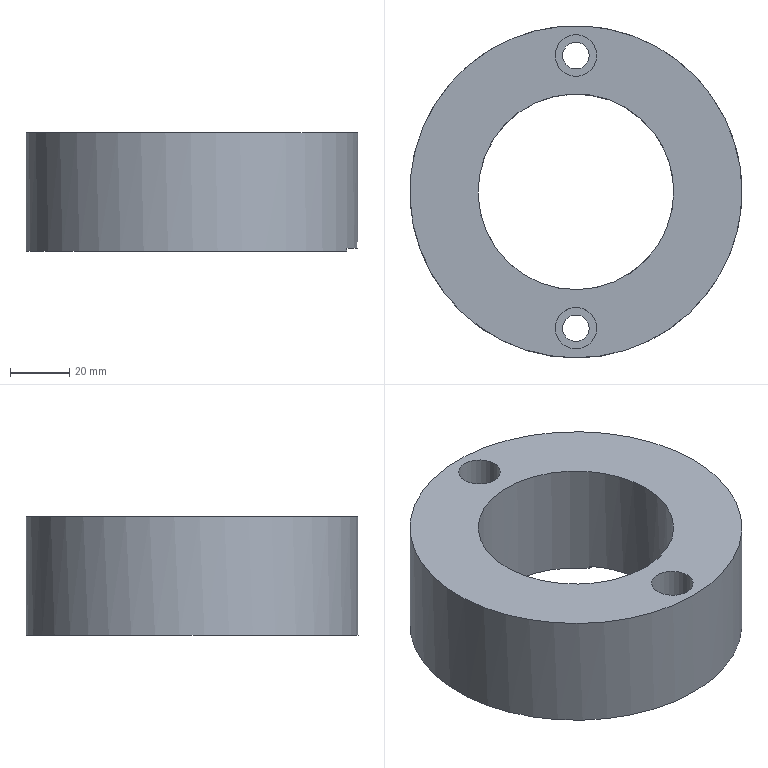Part | NX | features solid 2 | 1 solid | 13 faces | box 112 x 112 x 40 mm | volume 247574 mm3 | plane 7 | cylinder 6 | commonest cylinder face diameters 9 x2 14 x2 66 x1 112 x1
STEP:
#1=CARTESIAN_POINT('',(-633.751,-130.,-30.));
#2=VERTEX_POINT('',#1);
#3=CARTESIAN_POINT('',(-633.751,-130.,-29.));
#4=VERTEX_POINT('',#3);
#5=CARTESIAN_POINT('',(-633.751,-130.,20.));
#6=DIRECTION('',(0.,0.,-1.));
#7=VECTOR('',#6,1000.);
#8=LINE('',#5,#7);
#9=EDGE_CURVE('',#2,#4,#8,.F.);
#10=ORIENTED_EDGE('',*,*,#9,.T.);
#11=CARTESIAN_POINT('',(-633.751,-170.,-29.));
#12=VERTEX_POINT('',#11);
#13=CARTESIAN_POINT('',(-660.,-150.,-29.));
#14=DIRECTION('',(0.,0.,-1.));
#15=DIRECTION('',(1.,0.,0.));
#16=AXIS2_PLACEMENT_3D('',#13,#14,#15);
#17=CIRCLE('',#16,33.);
#18=EDGE_CURVE('',#4,#12,#17,.T.);
#19=ORIENTED_EDGE('',*,*,#18,.T.);
#20=CARTESIAN_POINT('',(-633.751,-170.,-30.));
#21=VERTEX_POINT('',#20);
#22=CARTESIAN_POINT('',(-633.751,-170.,20.));
#23=DIRECTION('',(0.,0.,-1.));
#24=VECTOR('',#23,1000.);
#25=LINE('',#22,#24);
#26=EDGE_CURVE('',#12,#21,#25,.T.);
#27=ORIENTED_EDGE('',*,*,#26,.T.);
#28=CARTESIAN_POINT('',(-660.,-150.,-30.));
#29=DIRECTION('',(0.,0.,-1.));
#30=DIRECTION('',(1.,0.,0.));
#31=AXIS2_PLACEMENT_3D('',#28,#29,#30);
#32=CIRCLE('',#31,33.);
#33=EDGE_CURVE('',#21,#2,#32,.T.);
#34=ORIENTED_EDGE('',*,*,#33,.T.);
#35=EDGE_LOOP('',(#10,#19,#27,#34));
#36=FACE_BOUND('',#35,.T.);
#37=CARTESIAN_POINT('',(-627.,-150.,10.));
#38=VERTEX_POINT('',#37);
#39=CARTESIAN_POINT('',(-660.,-150.,10.));
#40=DIRECTION('',(0.,0.,-1.));
#41=DIRECTION('',(1.,0.,0.));
#42=AXIS2_PLACEMENT_3D('',#39,#40,#41);
#43=CIRCLE('',#42,33.);
#44=EDGE_CURVE('',#38,#38,#43,.T.);
#45=ORIENTED_EDGE('',*,*,#44,.F.);
#46=EDGE_LOOP('',(#45));
#47=FACE_BOUND('',#46,.T.);
#48=CARTESIAN_POINT('',(-660.,-150.,20.));
#49=DIRECTION('',(0.,0.,-1.));
#50=DIRECTION('',(-1.,0.,0.));
#51=AXIS2_PLACEMENT_3D('',#48,#49,#50);
#52=CYLINDRICAL_SURFACE('',#51,33.);
#53=ADVANCED_FACE('',(#36,#47),#52,.F.);
#54=CARTESIAN_POINT('',(-604.,-150.,10.));
#55=VERTEX_POINT('',#54);
#56=CARTESIAN_POINT('',(-660.,-150.,10.));
#57=DIRECTION('',(0.,0.,-1.));
#58=DIRECTION('',(1.,0.,0.));
#59=AXIS2_PLACEMENT_3D('',#56,#57,#58);
#60=CIRCLE('',#59,56.);
#61=EDGE_CURVE('',#55,#55,#60,.T.);
#62=ORIENTED_EDGE('',*,*,#61,.T.);
#63=EDGE_LOOP('',(#62));
#64=FACE_BOUND('',#63,.T.);
#65=CARTESIAN_POINT('',(-607.693,-170.,-30.));
#66=VERTEX_POINT('',#65);
#67=CARTESIAN_POINT('',(-607.693,-130.,-30.));
#68=VERTEX_POINT('',#67);
#69=CARTESIAN_POINT('',(-660.,-150.,-30.));
#70=DIRECTION('',(0.,0.,-1.));
#71=DIRECTION('',(1.,0.,0.));
#72=AXIS2_PLACEMENT_3D('',#69,#70,#71);
#73=CIRCLE('',#72,56.);
#74=EDGE_CURVE('',#66,#68,#73,.T.);
#75=ORIENTED_EDGE('',*,*,#74,.F.);
#76=CARTESIAN_POINT('',(-607.693,-170.,-29.));
#77=VERTEX_POINT('',#76);
#78=CARTESIAN_POINT('',(-607.693,-170.,20.));
#79=DIRECTION('',(0.,0.,-1.));
#80=VECTOR('',#79,1000.);
#81=LINE('',#78,#80);
#82=EDGE_CURVE('',#77,#66,#81,.T.);
#83=ORIENTED_EDGE('',*,*,#82,.F.);
#84=CARTESIAN_POINT('',(-607.693,-130.,-29.));
#85=VERTEX_POINT('',#84);
#86=CARTESIAN_POINT('',(-660.,-150.,-29.));
#87=DIRECTION('',(0.,0.,-1.));
#88=DIRECTION('',(1.,0.,0.));
#89=AXIS2_PLACEMENT_3D('',#86,#87,#88);
#90=CIRCLE('',#89,56.);
#91=EDGE_CURVE('',#85,#77,#90,.T.);
#92=ORIENTED_EDGE('',*,*,#91,.F.);
#93=CARTESIAN_POINT('',(-607.693,-130.,20.));
#94=DIRECTION('',(0.,0.,-1.));
#95=VECTOR('',#94,1000.);
#96=LINE('',#93,#95);
#97=EDGE_CURVE('',#68,#85,#96,.F.);
#98=ORIENTED_EDGE('',*,*,#97,.F.);
#99=EDGE_LOOP('',(#75,#83,#92,#98));
#100=FACE_BOUND('',#99,.T.);
#101=CARTESIAN_POINT('',(-660.,-150.,20.));
#102=DIRECTION('',(0.,0.,-1.));
#103=DIRECTION('',(-1.,0.,0.));
#104=AXIS2_PLACEMENT_3D('',#101,#102,#103);
#105=CYLINDRICAL_SURFACE('',#104,56.);
#106=ADVANCED_FACE('',(#64,#100),#105,.T.);
#107=CARTESIAN_POINT('',(-653.,-104.,10.));
#108=VERTEX_POINT('',#107);
#109=CARTESIAN_POINT('',(-660.,-104.,10.));
#110=DIRECTION('',(0.,0.,-1.));
#111=DIRECTION('',(1.,0.,0.));
#112=AXIS2_PLACEMENT_3D('',#109,#110,#111);
#113=CIRCLE('',#112,7.);
#114=EDGE_CURVE('',#108,#108,#113,.F.);
#115=ORIENTED_EDGE('',*,*,#114,.F.);
#116=EDGE_LOOP('',(#115));
#117=FACE_BOUND('',#116,.T.);
#118=CARTESIAN_POINT('',(-653.,-196.,10.));
#119=VERTEX_POINT('',#118);
#120=CARTESIAN_POINT('',(-660.,-196.,10.));
#121=DIRECTION('',(0.,0.,-1.));
#122=DIRECTION('',(1.,0.,0.));
#123=AXIS2_PLACEMENT_3D('',#120,#121,#122);
#124=CIRCLE('',#123,7.);
#125=EDGE_CURVE('',#119,#119,#124,.F.);
#126=ORIENTED_EDGE('',*,*,#125,.F.);
#127=EDGE_LOOP('',(#126));
#128=FACE_BOUND('',#127,.T.);
#129=ORIENTED_EDGE('',*,*,#44,.T.);
#130=EDGE_LOOP('',(#129));
#131=FACE_BOUND('',#130,.T.);
#132=ORIENTED_EDGE('',*,*,#61,.F.);
#133=EDGE_LOOP('',(#132));
#134=FACE_BOUND('',#133,.T.);
#135=CARTESIAN_POINT('',(-660.,-150.,10.));
#136=DIRECTION('',(0.,0.,1.));
#137=DIRECTION('',(1.,0.,0.));
#138=AXIS2_PLACEMENT_3D('',#135,#136,#137);
#139=PLANE('',#138);
#140=ADVANCED_FACE('',(#117,#128,#131,#134),#139,.T.);
#141=CARTESIAN_POINT('',(-664.5,-104.,-30.));
#142=VERTEX_POINT('',#141);
#143=CARTESIAN_POINT('',(-660.,-104.,-30.));
#144=DIRECTION('',(0.,0.,1.));
#145=DIRECTION('',(-1.,0.,0.));
#146=AXIS2_PLACEMENT_3D('',#143,#144,#145);
#147=CIRCLE('',#146,4.5);
#148=EDGE_CURVE('',#142,#142,#147,.T.);
#149=ORIENTED_EDGE('',*,*,#148,.T.);
#150=EDGE_LOOP('',(#149));
#151=FACE_BOUND('',#150,.T.);
#152=CARTESIAN_POINT('',(-664.5,-196.,-30.));
#153=VERTEX_POINT('',#152);
#154=CARTESIAN_POINT('',(-660.,-196.,-30.));
#155=DIRECTION('',(0.,0.,1.));
#156=DIRECTION('',(-1.,0.,0.));
#157=AXIS2_PLACEMENT_3D('',#154,#155,#156);
#158=CIRCLE('',#157,4.5);
#159=EDGE_CURVE('',#153,#153,#158,.T.);
#160=ORIENTED_EDGE('',*,*,#159,.T.);
#161=EDGE_LOOP('',(#160));
#162=FACE_BOUND('',#161,.T.);
#163=ORIENTED_EDGE('',*,*,#33,.F.);
#164=CARTESIAN_POINT('',(-615.5,-170.,-30.));
#165=DIRECTION('',(1.,0.,0.));
#166=VECTOR('',#165,1000.);
#167=LINE('',#164,#166);
#168=EDGE_CURVE('',#21,#66,#167,.T.);
#169=ORIENTED_EDGE('',*,*,#168,.T.);
#170=ORIENTED_EDGE('',*,*,#74,.T.);
#171=CARTESIAN_POINT('',(-615.5,-130.,-30.));
#172=DIRECTION('',(1.,0.,0.));
#173=VECTOR('',#172,1000.);
#174=LINE('',#171,#173);
#175=EDGE_CURVE('',#2,#68,#174,.T.);
#176=ORIENTED_EDGE('',*,*,#175,.F.);
#177=EDGE_LOOP('',(#163,#169,#170,#176));
#178=FACE_BOUND('',#177,.T.);
#179=CARTESIAN_POINT('',(-660.,-150.,-30.));
#180=DIRECTION('',(0.,0.,1.));
#181=DIRECTION('',(1.,0.,0.));
#182=AXIS2_PLACEMENT_3D('',#179,#180,#181);
#183=PLANE('',#182);
#184=ADVANCED_FACE('',(#151,#162,#178),#183,.F.);
#185=ORIENTED_EDGE('',*,*,#159,.F.);
#186=EDGE_LOOP('',(#185));
#187=FACE_BOUND('',#186,.T.);
#188=CARTESIAN_POINT('',(-664.5,-196.,-10.));
#189=VERTEX_POINT('',#188);
#190=CARTESIAN_POINT('',(-660.,-196.,-10.));
#191=DIRECTION('',(0.,0.,1.));
#192=DIRECTION('',(-1.,0.,0.));
#193=AXIS2_PLACEMENT_3D('',#190,#191,#192);
#194=CIRCLE('',#193,4.5);
#195=EDGE_CURVE('',#189,#189,#194,.T.);
#196=ORIENTED_EDGE('',*,*,#195,.T.);
#197=EDGE_LOOP('',(#196));
#198=FACE_BOUND('',#197,.T.);
#199=CARTESIAN_POINT('',(-660.,-196.,-30.));
#200=DIRECTION('',(0.,0.,-1.));
#201=DIRECTION('',(-1.,0.,0.));
#202=AXIS2_PLACEMENT_3D('',#199,#200,#201);
#203=CYLINDRICAL_SURFACE('',#202,4.5);
#204=ADVANCED_FACE('',(#187,#198),#203,.F.);
#205=ORIENTED_EDGE('',*,*,#195,.F.);
#206=EDGE_LOOP('',(#205));
#207=FACE_BOUND('',#206,.T.);
#208=CARTESIAN_POINT('',(-667.,-196.,-10.));
#209=VERTEX_POINT('',#208);
#210=CARTESIAN_POINT('',(-660.,-196.,-10.));
#211=DIRECTION('',(0.,0.,1.));
#212=DIRECTION('',(-1.,0.,0.));
#213=AXIS2_PLACEMENT_3D('',#210,#211,#212);
#214=CIRCLE('',#213,7.);
#215=EDGE_CURVE('',#209,#209,#214,.T.);
#216=ORIENTED_EDGE('',*,*,#215,.T.);
#217=EDGE_LOOP('',(#216));
#218=FACE_BOUND('',#217,.T.);
#219=CARTESIAN_POINT('',(-660.,-196.,-10.));
#220=DIRECTION('',(0.,0.,-1.));
#221=DIRECTION('',(-1.,0.,0.));
#222=AXIS2_PLACEMENT_3D('',#219,#220,#221);
#223=PLANE('',#222);
#224=ADVANCED_FACE('',(#207,#218),#223,.F.);
#225=ORIENTED_EDGE('',*,*,#215,.F.);
#226=EDGE_LOOP('',(#225));
#227=FACE_BOUND('',#226,.T.);
#228=ORIENTED_EDGE('',*,*,#125,.T.);
#229=EDGE_LOOP('',(#228));
#230=FACE_BOUND('',#229,.T.);
#231=CARTESIAN_POINT('',(-660.,-196.,20.));
#232=DIRECTION('',(0.,0.,-1.));
#233=DIRECTION('',(-1.,0.,0.));
#234=AXIS2_PLACEMENT_3D('',#231,#232,#233);
#235=CYLINDRICAL_SURFACE('',#234,7.);
#236=ADVANCED_FACE('',(#227,#230),#235,.F.);
#237=ORIENTED_EDGE('',*,*,#148,.F.);
#238=EDGE_LOOP('',(#237));
#239=FACE_BOUND('',#238,.T.);
#240=CARTESIAN_POINT('',(-664.5,-104.,-10.));
#241=VERTEX_POINT('',#240);
#242=CARTESIAN_POINT('',(-660.,-104.,-10.));
#243=DIRECTION('',(0.,0.,1.));
#244=DIRECTION('',(-1.,0.,0.));
#245=AXIS2_PLACEMENT_3D('',#242,#243,#244);
#246=CIRCLE('',#245,4.5);
#247=EDGE_CURVE('',#241,#241,#246,.T.);
#248=ORIENTED_EDGE('',*,*,#247,.T.);
#249=EDGE_LOOP('',(#248));
#250=FACE_BOUND('',#249,.T.);
#251=CARTESIAN_POINT('',(-660.,-104.,-30.));
#252=DIRECTION('',(0.,0.,-1.));
#253=DIRECTION('',(-1.,0.,0.));
#254=AXIS2_PLACEMENT_3D('',#251,#252,#253);
#255=CYLINDRICAL_SURFACE('',#254,4.5);
#256=ADVANCED_FACE('',(#239,#250),#255,.F.);
#257=ORIENTED_EDGE('',*,*,#247,.F.);
#258=EDGE_LOOP('',(#257));
#259=FACE_BOUND('',#258,.T.);
#260=CARTESIAN_POINT('',(-667.,-104.,-10.));
#261=VERTEX_POINT('',#260);
#262=CARTESIAN_POINT('',(-660.,-104.,-10.));
#263=DIRECTION('',(0.,0.,1.));
#264=DIRECTION('',(-1.,0.,0.));
#265=AXIS2_PLACEMENT_3D('',#262,#263,#264);
#266=CIRCLE('',#265,7.);
#267=EDGE_CURVE('',#261,#261,#266,.T.);
#268=ORIENTED_EDGE('',*,*,#267,.T.);
#269=EDGE_LOOP('',(#268));
#270=FACE_BOUND('',#269,.T.);
#271=CARTESIAN_POINT('',(-660.,-104.,-10.));
#272=DIRECTION('',(0.,0.,-1.));
#273=DIRECTION('',(-1.,0.,0.));
#274=AXIS2_PLACEMENT_3D('',#271,#272,#273);
#275=PLANE('',#274);
#276=ADVANCED_FACE('',(#259,#270),#275,.F.);
#277=ORIENTED_EDGE('',*,*,#267,.F.);
#278=EDGE_LOOP('',(#277));
#279=FACE_BOUND('',#278,.T.);
#280=ORIENTED_EDGE('',*,*,#114,.T.);
#281=EDGE_LOOP('',(#280));
#282=FACE_BOUND('',#281,.T.);
#283=CARTESIAN_POINT('',(-660.,-104.,20.));
#284=DIRECTION('',(0.,0.,-1.));
#285=DIRECTION('',(-1.,0.,0.));
#286=AXIS2_PLACEMENT_3D('',#283,#284,#285);
#287=CYLINDRICAL_SURFACE('',#286,7.);
#288=ADVANCED_FACE('',(#279,#282),#287,.F.);
#289=ORIENTED_EDGE('',*,*,#18,.F.);
#290=CARTESIAN_POINT('',(-638.5,-130.,-29.));
#291=DIRECTION('',(1.,0.,0.));
#292=VECTOR('',#291,1000.);
#293=LINE('',#290,#292);
#294=EDGE_CURVE('',#4,#85,#293,.T.);
#295=ORIENTED_EDGE('',*,*,#294,.T.);
#296=ORIENTED_EDGE('',*,*,#91,.T.);
#297=CARTESIAN_POINT('',(-638.5,-170.,-29.));
#298=DIRECTION('',(1.,0.,0.));
#299=VECTOR('',#298,1000.);
#300=LINE('',#297,#299);
#301=EDGE_CURVE('',#12,#77,#300,.T.);
#302=ORIENTED_EDGE('',*,*,#301,.F.);
#303=EDGE_LOOP('',(#289,#295,#296,#302));
#304=FACE_BOUND('',#303,.T.);
#305=CARTESIAN_POINT('',(-615.5,-150.,-29.));
#306=DIRECTION('',(0.,0.,1.));
#307=DIRECTION('',(1.,0.,0.));
#308=AXIS2_PLACEMENT_3D('',#305,#306,#307);
#309=PLANE('',#308);
#310=ADVANCED_FACE('',(#304),#309,.F.);
#311=ORIENTED_EDGE('',*,*,#9,.F.);
#312=ORIENTED_EDGE('',*,*,#175,.T.);
#313=ORIENTED_EDGE('',*,*,#97,.T.);
#314=ORIENTED_EDGE('',*,*,#294,.F.);
#315=EDGE_LOOP('',(#311,#312,#313,#314));
#316=FACE_BOUND('',#315,.T.);
#317=CARTESIAN_POINT('',(-615.5,-130.,-30.));
#318=DIRECTION('',(0.,1.,0.));
#319=DIRECTION('',(0.,0.,-1.));
#320=AXIS2_PLACEMENT_3D('',#317,#318,#319);
#321=PLANE('',#320);
#322=ADVANCED_FACE('',(#316),#321,.F.);
#323=ORIENTED_EDGE('',*,*,#26,.F.);
#324=ORIENTED_EDGE('',*,*,#301,.T.);
#325=ORIENTED_EDGE('',*,*,#82,.T.);
#326=ORIENTED_EDGE('',*,*,#168,.F.);
#327=EDGE_LOOP('',(#323,#324,#325,#326));
#328=FACE_BOUND('',#327,.T.);
#329=CARTESIAN_POINT('',(-615.5,-170.,-30.));
#330=DIRECTION('',(0.,-1.,0.));
#331=DIRECTION('',(0.,0.,1.));
#332=AXIS2_PLACEMENT_3D('',#329,#330,#331);
#333=PLANE('',#332);
#334=ADVANCED_FACE('',(#328),#333,.F.);
#335=CLOSED_SHELL('',(#53,#106,#140,#184,#204,#224,#236,#256,#276,#288,#310,#322,#334));
#336=MANIFOLD_SOLID_BREP('',#335);
#337=(LENGTH_UNIT()NAMED_UNIT(*)SI_UNIT(.MILLI.,.METRE.));
#338=UNCERTAINTY_MEASURE_WITH_UNIT(LENGTH_MEASURE(0.00001),#337,'','');
#339=(NAMED_UNIT(*)PLANE_ANGLE_UNIT()SI_UNIT($,.RADIAN.));
#340=(NAMED_UNIT(*)SI_UNIT($,.STERADIAN.)SOLID_ANGLE_UNIT());
#341=(GEOMETRIC_REPRESENTATION_CONTEXT(3)GLOBAL_UNCERTAINTY_ASSIGNED_CONTEXT((#338))GLOBAL_UNIT_ASSIGNED_CONTEXT((#337,#339,#340))REPRESENTATION_CONTEXT('',''));
#342=ADVANCED_BREP_SHAPE_REPRESENTATION('',(#336),#341);